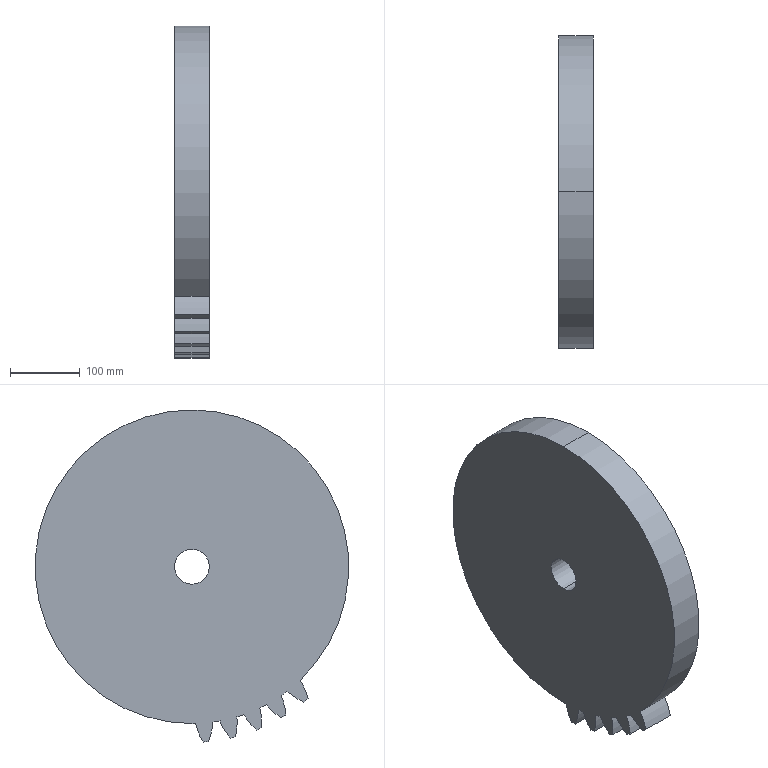Part | SolidWorks | features ICE 2, BaseBody 1 | 1 solid | 26 faces | box 50 x 449.998 x 476.498 mm | volume 7974553 mm3 | cylinder 24 | plane 2 | commonest cylinder face diameters 192 x10 449.998 x7 504 x5 50 x2
STEP:
#1=CARTESIAN_POINT('',(50.,0.,25.));
#2=VERTEX_POINT('',#1);
#3=CARTESIAN_POINT('',(50.,0.,-25.));
#4=VERTEX_POINT('',#3);
#5=CARTESIAN_POINT('',(50.,0.,0.));
#6=DIRECTION('',(1.,0.,0.));
#7=DIRECTION('',(0.,0.,1.));
#8=AXIS2_PLACEMENT_3D('',#5,#6,#7);
#9=CIRCLE('',#8,25.);
#10=EDGE_CURVE('',#2,#4,#9,.T.);
#11=ORIENTED_EDGE('',*,*,#10,.T.);
#12=CARTESIAN_POINT('',(0.,0.,-25.));
#13=VERTEX_POINT('',#12);
#14=CARTESIAN_POINT('',(50.,0.,-25.));
#15=DIRECTION('',(-1.,0.,0.));
#16=VECTOR('',#15,1000.);
#17=LINE('',#14,#16);
#18=EDGE_CURVE('',#4,#13,#17,.T.);
#19=ORIENTED_EDGE('',*,*,#18,.T.);
#20=CARTESIAN_POINT('',(0.,0.,25.));
#21=VERTEX_POINT('',#20);
#22=CARTESIAN_POINT('',(0.,0.,0.));
#23=DIRECTION('',(-1.,0.,0.));
#24=DIRECTION('',(0.,0.,1.));
#25=AXIS2_PLACEMENT_3D('',#22,#23,#24);
#26=CIRCLE('',#25,25.);
#27=EDGE_CURVE('',#13,#21,#26,.T.);
#28=ORIENTED_EDGE('',*,*,#27,.T.);
#29=CARTESIAN_POINT('',(50.,0.,25.));
#30=DIRECTION('',(-1.,0.,0.));
#31=VECTOR('',#30,1000.);
#32=LINE('',#29,#31);
#33=EDGE_CURVE('',#2,#21,#32,.T.);
#34=ORIENTED_EDGE('',*,*,#33,.F.);
#35=EDGE_LOOP('',(#11,#19,#28,#34));
#36=FACE_OUTER_BOUND('',#35,.T.);
#37=CARTESIAN_POINT('',(50.,0.,0.));
#38=DIRECTION('',(-1.,0.,0.));
#39=DIRECTION('',(0.,0.,1.));
#40=AXIS2_PLACEMENT_3D('',#37,#38,#39);
#41=CYLINDRICAL_SURFACE('',#40,25.);
#42=ADVANCED_FACE('',(#36),#41,.F.);
#43=CARTESIAN_POINT('',(50.,0.,224.999));
#44=VERTEX_POINT('',#43);
#45=CARTESIAN_POINT('',(50.,0.,-224.999));
#46=VERTEX_POINT('',#45);
#47=CARTESIAN_POINT('',(50.,0.,0.));
#48=DIRECTION('',(-1.,0.,0.));
#49=DIRECTION('',(0.,0.,-1.));
#50=AXIS2_PLACEMENT_3D('',#47,#48,#49);
#51=CIRCLE('',#50,224.999);
#52=EDGE_CURVE('',#44,#46,#51,.T.);
#53=ORIENTED_EDGE('',*,*,#52,.T.);
#54=CARTESIAN_POINT('',(0.,0.,-224.999));
#55=VERTEX_POINT('',#54);
#56=CARTESIAN_POINT('',(50.,0.,-224.999));
#57=DIRECTION('',(-1.,0.,0.));
#58=VECTOR('',#57,1000.);
#59=LINE('',#56,#58);
#60=EDGE_CURVE('',#46,#55,#59,.T.);
#61=ORIENTED_EDGE('',*,*,#60,.T.);
#62=CARTESIAN_POINT('',(0.,0.,224.999));
#63=VERTEX_POINT('',#62);
#64=CARTESIAN_POINT('',(0.,0.,0.));
#65=DIRECTION('',(-1.,0.,0.));
#66=DIRECTION('',(0.,0.,-1.));
#67=AXIS2_PLACEMENT_3D('',#64,#65,#66);
#68=CIRCLE('',#67,224.999);
#69=EDGE_CURVE('',#63,#55,#68,.T.);
#70=ORIENTED_EDGE('',*,*,#69,.F.);
#71=CARTESIAN_POINT('',(50.,0.,224.999));
#72=DIRECTION('',(-1.,0.,0.));
#73=VECTOR('',#72,1000.);
#74=LINE('',#71,#73);
#75=EDGE_CURVE('',#44,#63,#74,.T.);
#76=ORIENTED_EDGE('',*,*,#75,.F.);
#77=EDGE_LOOP('',(#53,#61,#70,#76));
#78=FACE_OUTER_BOUND('',#77,.T.);
#79=CARTESIAN_POINT('',(50.,0.,0.));
#80=DIRECTION('',(-1.,0.,0.));
#81=DIRECTION('',(0.,0.,1.));
#82=AXIS2_PLACEMENT_3D('',#79,#80,#81);
#83=CYLINDRICAL_SURFACE('',#82,224.999);
#84=ADVANCED_FACE('',(#78),#83,.T.);
#85=CARTESIAN_POINT('',(50.,-155.378,-162.734));
#86=VERTEX_POINT('',#85);
#87=CARTESIAN_POINT('',(50.,0.,0.));
#88=DIRECTION('',(-1.,0.,0.));
#89=DIRECTION('',(0.,0.,-1.));
#90=AXIS2_PLACEMENT_3D('',#87,#88,#89);
#91=CIRCLE('',#90,224.999);
#92=EDGE_CURVE('',#86,#44,#91,.T.);
#93=ORIENTED_EDGE('',*,*,#92,.T.);
#94=ORIENTED_EDGE('',*,*,#75,.T.);
#95=CARTESIAN_POINT('',(0.,-155.378,-162.734));
#96=VERTEX_POINT('',#95);
#97=CARTESIAN_POINT('',(0.,0.,0.));
#98=DIRECTION('',(-1.,0.,0.));
#99=DIRECTION('',(0.,0.,-1.));
#100=AXIS2_PLACEMENT_3D('',#97,#98,#99);
#101=CIRCLE('',#100,224.999);
#102=EDGE_CURVE('',#96,#63,#101,.T.);
#103=ORIENTED_EDGE('',*,*,#102,.F.);
#104=CARTESIAN_POINT('',(50.,-155.378,-162.734));
#105=DIRECTION('',(-1.,0.,0.));
#106=VECTOR('',#105,1000.);
#107=LINE('',#104,#106);
#108=EDGE_CURVE('',#86,#96,#107,.T.);
#109=ORIENTED_EDGE('',*,*,#108,.F.);
#110=EDGE_LOOP('',(#93,#94,#103,#109));
#111=FACE_OUTER_BOUND('',#110,.T.);
#112=CARTESIAN_POINT('',(50.,0.,0.));
#113=DIRECTION('',(-1.,0.,0.));
#114=DIRECTION('',(0.,0.,1.));
#115=AXIS2_PLACEMENT_3D('',#112,#113,#114);
#116=CYLINDRICAL_SURFACE('',#115,224.999);
#117=ADVANCED_FACE('',(#111),#116,.T.);
#118=ORIENTED_EDGE('',*,*,#10,.F.);
#119=CARTESIAN_POINT('',(50.,0.,0.));
#120=DIRECTION('',(1.,0.,0.));
#121=DIRECTION('',(0.,0.,1.));
#122=AXIS2_PLACEMENT_3D('',#119,#120,#121);
#123=CIRCLE('',#122,25.);
#124=EDGE_CURVE('',#4,#2,#123,.T.);
#125=ORIENTED_EDGE('',*,*,#124,.F.);
#126=EDGE_LOOP('',(#118,#125));
#127=FACE_BOUND('',#126,.T.);
#128=ORIENTED_EDGE('',*,*,#92,.F.);
#129=CARTESIAN_POINT('',(50.,-166.611,-189.062));
#130=VERTEX_POINT('',#129);
#131=CARTESIAN_POINT('',(50.,-73.683,-213.15));
#132=DIRECTION('',(-1.,0.,0.));
#133=DIRECTION('',(0.,-0.7071,0.7071));
#134=AXIS2_PLACEMENT_3D('',#131,#132,#133);
#135=CIRCLE('',#134,96.);
#136=EDGE_CURVE('',#130,#86,#135,.T.);
#137=ORIENTED_EDGE('',*,*,#136,.F.);
#138=CARTESIAN_POINT('',(50.,-160.671,-194.136));
#139=VERTEX_POINT('',#138);
#140=CARTESIAN_POINT('',(50.,0.,0.));
#141=DIRECTION('',(-1.,0.,0.));
#142=DIRECTION('',(0.,0.,1.));
#143=AXIS2_PLACEMENT_3D('',#140,#141,#142);
#144=CIRCLE('',#143,252.);
#145=EDGE_CURVE('',#139,#130,#144,.T.);
#146=ORIENTED_EDGE('',*,*,#145,.F.);
#147=CARTESIAN_POINT('',(50.,-136.423,-178.922));
#148=VERTEX_POINT('',#147);
#149=CARTESIAN_POINT('',(50.,-198.999,-106.119));
#150=DIRECTION('',(-1.,0.,0.));
#151=DIRECTION('',(0.,-0.809,0.5878));
#152=AXIS2_PLACEMENT_3D('',#149,#150,#151);
#153=CIRCLE('',#152,96.);
#154=EDGE_CURVE('',#148,#139,#153,.T.);
#155=ORIENTED_EDGE('',*,*,#154,.F.);
#156=CARTESIAN_POINT('',(50.,-128.008,-185.036));
#157=VERTEX_POINT('',#156);
#158=CARTESIAN_POINT('',(50.,0.,0.));
#159=DIRECTION('',(-1.,0.,0.));
#160=DIRECTION('',(0.,-0.809,0.5878));
#161=AXIS2_PLACEMENT_3D('',#158,#159,#160);
#162=CIRCLE('',#161,224.999);
#163=EDGE_CURVE('',#157,#148,#162,.T.);
#164=ORIENTED_EDGE('',*,*,#163,.F.);
#165=CARTESIAN_POINT('',(50.,-134.984,-212.799));
#166=VERTEX_POINT('',#165);
#167=CARTESIAN_POINT('',(50.,-39.431,-222.052));
#168=DIRECTION('',(-1.,0.,0.));
#169=DIRECTION('',(0.,-0.809,0.5878));
#170=AXIS2_PLACEMENT_3D('',#167,#168,#169);
#171=CIRCLE('',#170,96.);
#172=EDGE_CURVE('',#166,#157,#171,.T.);
#173=ORIENTED_EDGE('',*,*,#172,.F.);
#174=CARTESIAN_POINT('',(50.,-128.323,-216.88));
#175=VERTEX_POINT('',#174);
#176=CARTESIAN_POINT('',(50.,0.,0.));
#177=DIRECTION('',(-1.,0.,0.));
#178=DIRECTION('',(0.,0.,1.));
#179=AXIS2_PLACEMENT_3D('',#176,#177,#178);
#180=CIRCLE('',#179,252.);
#181=EDGE_CURVE('',#175,#166,#180,.T.);
#182=ORIENTED_EDGE('',*,*,#181,.F.);
#183=CARTESIAN_POINT('',(50.,-106.754,-198.061));
#184=VERTEX_POINT('',#183);
#185=CARTESIAN_POINT('',(50.,-179.949,-135.943));
#186=DIRECTION('',(-1.,0.,0.));
#187=DIRECTION('',(0.,-0.891,0.454));
#188=AXIS2_PLACEMENT_3D('',#185,#186,#187);
#189=CIRCLE('',#188,96.);
#190=EDGE_CURVE('',#184,#175,#189,.T.);
#191=ORIENTED_EDGE('',*,*,#190,.F.);
#192=CARTESIAN_POINT('',(50.,-97.486,-202.783));
#193=VERTEX_POINT('',#192);
#194=CARTESIAN_POINT('',(50.,0.,0.));
#195=DIRECTION('',(-1.,0.,0.));
#196=DIRECTION('',(0.,-0.891,0.454));
#197=AXIS2_PLACEMENT_3D('',#194,#195,#196);
#198=CIRCLE('',#197,224.999);
#199=EDGE_CURVE('',#193,#184,#198,.T.);
#200=ORIENTED_EDGE('',*,*,#199,.F.);
#201=CARTESIAN_POINT('',(50.,-100.033,-231.295));
#202=VERTEX_POINT('',#201);
#203=CARTESIAN_POINT('',(50.,-4.209,-225.487));
#204=DIRECTION('',(-1.,0.,0.));
#205=DIRECTION('',(0.,-0.891,0.454));
#206=AXIS2_PLACEMENT_3D('',#203,#204,#205);
#207=CIRCLE('',#206,96.);
#208=EDGE_CURVE('',#202,#193,#207,.T.);
#209=ORIENTED_EDGE('',*,*,#208,.F.);
#210=CARTESIAN_POINT('',(50.,-92.816,-234.284));
#211=VERTEX_POINT('',#210);
#212=CARTESIAN_POINT('',(50.,0.,0.));
#213=DIRECTION('',(-1.,0.,0.));
#214=DIRECTION('',(0.,0.,1.));
#215=AXIS2_PLACEMENT_3D('',#212,#213,#214);
#216=CIRCLE('',#215,252.);
#217=EDGE_CURVE('',#211,#202,#216,.T.);
#218=ORIENTED_EDGE('',*,*,#217,.F.);
#219=CARTESIAN_POINT('',(50.,-74.456,-212.322));
#220=VERTEX_POINT('',#219);
#221=CARTESIAN_POINT('',(50.,-156.467,-162.42));
#222=DIRECTION('',(-1.,0.,0.));
#223=DIRECTION('',(0.,-0.9511,0.309));
#224=AXIS2_PLACEMENT_3D('',#221,#222,#223);
#225=CIRCLE('',#224,96.);
#226=EDGE_CURVE('',#220,#211,#225,.T.);
#227=ORIENTED_EDGE('',*,*,#226,.F.);
#228=CARTESIAN_POINT('',(50.,-64.563,-215.537));
#229=VERTEX_POINT('',#228);
#230=CARTESIAN_POINT('',(50.,0.,0.));
#231=DIRECTION('',(-1.,0.,0.));
#232=DIRECTION('',(0.,-0.9511,0.309));
#233=AXIS2_PLACEMENT_3D('',#230,#231,#232);
#234=CIRCLE('',#233,224.999);
#235=EDGE_CURVE('',#229,#220,#234,.T.);
#236=ORIENTED_EDGE('',*,*,#235,.F.);
#237=CARTESIAN_POINT('',(50.,-62.619,-244.096));
#238=VERTEX_POINT('',#237);
#239=CARTESIAN_POINT('',(50.,31.117,-223.369));
#240=DIRECTION('',(-1.,0.,0.));
#241=DIRECTION('',(0.,-0.9511,0.309));
#242=AXIS2_PLACEMENT_3D('',#239,#240,#241);
#243=CIRCLE('',#242,96.);
#244=EDGE_CURVE('',#238,#229,#243,.T.);
#245=ORIENTED_EDGE('',*,*,#244,.F.);
#246=CARTESIAN_POINT('',(50.,-55.023,-245.92));
#247=VERTEX_POINT('',#246);
#248=CARTESIAN_POINT('',(50.,0.,0.));
#249=DIRECTION('',(-1.,0.,0.));
#250=DIRECTION('',(0.,0.,1.));
#251=AXIS2_PLACEMENT_3D('',#248,#249,#250);
#252=CIRCLE('',#251,252.);
#253=EDGE_CURVE('',#247,#238,#252,.T.);
#254=ORIENTED_EDGE('',*,*,#253,.F.);
#255=CARTESIAN_POINT('',(50.,-40.325,-221.356));
#256=VERTEX_POINT('',#255);
#257=CARTESIAN_POINT('',(50.,-129.133,-184.897));
#258=DIRECTION('',(-1.,0.,0.));
#259=DIRECTION('',(0.,-0.9877,0.1564));
#260=AXIS2_PLACEMENT_3D('',#257,#258,#259);
#261=CIRCLE('',#260,96.);
#262=EDGE_CURVE('',#256,#247,#261,.T.);
#263=ORIENTED_EDGE('',*,*,#262,.F.);
#264=CARTESIAN_POINT('',(50.,-30.051,-222.983));
#265=VERTEX_POINT('',#264);
#266=CARTESIAN_POINT('',(50.,0.,0.));
#267=DIRECTION('',(-1.,0.,0.));
#268=DIRECTION('',(0.,-0.9877,0.1564));
#269=AXIS2_PLACEMENT_3D('',#266,#267,#268);
#270=CIRCLE('',#269,224.999);
#271=EDGE_CURVE('',#265,#256,#270,.T.);
#272=ORIENTED_EDGE('',*,*,#271,.F.);
#273=CARTESIAN_POINT('',(50.,-23.663,-250.887));
#274=VERTEX_POINT('',#273);
#275=CARTESIAN_POINT('',(50.,65.676,-215.752));
#276=DIRECTION('',(-1.,0.,0.));
#277=DIRECTION('',(0.,-0.9877,0.1564));
#278=AXIS2_PLACEMENT_3D('',#275,#276,#277);
#279=CIRCLE('',#278,96.);
#280=EDGE_CURVE('',#274,#265,#279,.T.);
#281=ORIENTED_EDGE('',*,*,#280,.F.);
#282=CARTESIAN_POINT('',(50.,-15.875,-251.499));
#283=VERTEX_POINT('',#282);
#284=CARTESIAN_POINT('',(50.,0.,0.));
#285=DIRECTION('',(-1.,0.,0.));
#286=DIRECTION('',(0.,0.,1.));
#287=AXIS2_PLACEMENT_3D('',#284,#285,#286);
#288=CIRCLE('',#287,252.);
#289=EDGE_CURVE('',#283,#274,#288,.T.);
#290=ORIENTED_EDGE('',*,*,#289,.F.);
#291=CARTESIAN_POINT('',(50.,-5.201,-224.939));
#292=VERTEX_POINT('',#291);
#293=CARTESIAN_POINT('',(50.,-98.618,-202.821));
#294=DIRECTION('',(-1.,0.,0.));
#295=DIRECTION('',(0.,-1.,0.));
#296=AXIS2_PLACEMENT_3D('',#293,#294,#295);
#297=CIRCLE('',#296,96.);
#298=EDGE_CURVE('',#292,#283,#297,.T.);
#299=ORIENTED_EDGE('',*,*,#298,.F.);
#300=CARTESIAN_POINT('',(50.,0.,0.));
#301=DIRECTION('',(-1.,0.,0.));
#302=DIRECTION('',(0.,0.,-1.));
#303=AXIS2_PLACEMENT_3D('',#300,#301,#302);
#304=CIRCLE('',#303,224.999);
#305=EDGE_CURVE('',#46,#292,#304,.T.);
#306=ORIENTED_EDGE('',*,*,#305,.F.);
#307=ORIENTED_EDGE('',*,*,#52,.F.);
#308=EDGE_LOOP('',(#128,#137,#146,#155,#164,#173,#182,#191,#200,#209,#218,#227,#236,#245,#254,#263,#272,#281,#290,#299,#306,#307));
#309=FACE_OUTER_BOUND('',#308,.T.);
#310=CARTESIAN_POINT('',(50.,0.,0.));
#311=DIRECTION('',(-1.,0.,0.));
#312=DIRECTION('',(0.,0.,1.));
#313=AXIS2_PLACEMENT_3D('',#310,#311,#312);
#314=PLANE('',#313);
#315=ADVANCED_FACE('',(#127,#309),#314,.F.);
#316=CARTESIAN_POINT('',(0.,-160.671,-194.136));
#317=VERTEX_POINT('',#316);
#318=CARTESIAN_POINT('',(25.,-160.671,-194.136));
#319=DIRECTION('',(-1.,0.,0.));
#320=VECTOR('',#319,1000.);
#321=LINE('',#318,#320);
#322=EDGE_CURVE('',#139,#317,#321,.T.);
#323=ORIENTED_EDGE('',*,*,#322,.F.);
#324=ORIENTED_EDGE('',*,*,#145,.T.);
#325=CARTESIAN_POINT('',(0.,-166.611,-189.062));
#326=VERTEX_POINT('',#325);
#327=CARTESIAN_POINT('',(25.,-166.611,-189.062));
#328=DIRECTION('',(1.,0.,0.));
#329=VECTOR('',#328,1000.);
#330=LINE('',#327,#329);
#331=EDGE_CURVE('',#326,#130,#330,.T.);
#332=ORIENTED_EDGE('',*,*,#331,.F.);
#333=CARTESIAN_POINT('',(0.,0.,0.));
#334=DIRECTION('',(-1.,0.,0.));
#335=DIRECTION('',(0.,0.,1.));
#336=AXIS2_PLACEMENT_3D('',#333,#334,#335);
#337=CIRCLE('',#336,252.);
#338=EDGE_CURVE('',#317,#326,#337,.T.);
#339=ORIENTED_EDGE('',*,*,#338,.F.);
#340=EDGE_LOOP('',(#323,#324,#332,#339));
#341=FACE_OUTER_BOUND('',#340,.T.);
#342=CARTESIAN_POINT('',(-10.,0.,0.));
#343=DIRECTION('',(-1.,0.,0.));
#344=DIRECTION('',(0.,0.,1.));
#345=AXIS2_PLACEMENT_3D('',#342,#343,#344);
#346=CYLINDRICAL_SURFACE('',#345,252.);
#347=ADVANCED_FACE('',(#341),#346,.T.);
#348=CARTESIAN_POINT('',(0.,-134.984,-212.799));
#349=VERTEX_POINT('',#348);
#350=CARTESIAN_POINT('',(25.,-134.984,-212.799));
#351=DIRECTION('',(1.,0.,0.));
#352=VECTOR('',#351,1000.);
#353=LINE('',#350,#352);
#354=EDGE_CURVE('',#349,#166,#353,.T.);
#355=ORIENTED_EDGE('',*,*,#354,.F.);
#356=CARTESIAN_POINT('',(0.,-128.323,-216.88));
#357=VERTEX_POINT('',#356);
#358=CARTESIAN_POINT('',(0.,0.,0.));
#359=DIRECTION('',(-1.,0.,0.));
#360=DIRECTION('',(0.,0.,1.));
#361=AXIS2_PLACEMENT_3D('',#358,#359,#360);
#362=CIRCLE('',#361,252.);
#363=EDGE_CURVE('',#357,#349,#362,.T.);
#364=ORIENTED_EDGE('',*,*,#363,.F.);
#365=CARTESIAN_POINT('',(25.,-128.323,-216.88));
#366=DIRECTION('',(-1.,0.,0.));
#367=VECTOR('',#366,1000.);
#368=LINE('',#365,#367);
#369=EDGE_CURVE('',#175,#357,#368,.T.);
#370=ORIENTED_EDGE('',*,*,#369,.F.);
#371=ORIENTED_EDGE('',*,*,#181,.T.);
#372=EDGE_LOOP('',(#355,#364,#370,#371));
#373=FACE_OUTER_BOUND('',#372,.T.);
#374=CARTESIAN_POINT('',(-10.,0.,0.));
#375=DIRECTION('',(-1.,0.,0.));
#376=DIRECTION('',(0.,0.,1.));
#377=AXIS2_PLACEMENT_3D('',#374,#375,#376);
#378=CYLINDRICAL_SURFACE('',#377,252.);
#379=ADVANCED_FACE('',(#373),#378,.T.);
#380=CARTESIAN_POINT('',(0.,-100.033,-231.295));
#381=VERTEX_POINT('',#380);
#382=CARTESIAN_POINT('',(25.,-100.033,-231.295));
#383=DIRECTION('',(1.,0.,0.));
#384=VECTOR('',#383,1000.);
#385=LINE('',#382,#384);
#386=EDGE_CURVE('',#381,#202,#385,.T.);
#387=ORIENTED_EDGE('',*,*,#386,.F.);
#388=CARTESIAN_POINT('',(0.,-92.816,-234.284));
#389=VERTEX_POINT('',#388);
#390=CARTESIAN_POINT('',(0.,0.,0.));
#391=DIRECTION('',(-1.,0.,0.));
#392=DIRECTION('',(0.,0.,1.));
#393=AXIS2_PLACEMENT_3D('',#390,#391,#392);
#394=CIRCLE('',#393,252.);
#395=EDGE_CURVE('',#389,#381,#394,.T.);
#396=ORIENTED_EDGE('',*,*,#395,.F.);
#397=CARTESIAN_POINT('',(25.,-92.816,-234.284));
#398=DIRECTION('',(-1.,0.,0.));
#399=VECTOR('',#398,1000.);
#400=LINE('',#397,#399);
#401=EDGE_CURVE('',#211,#389,#400,.T.);
#402=ORIENTED_EDGE('',*,*,#401,.F.);
#403=ORIENTED_EDGE('',*,*,#217,.T.);
#404=EDGE_LOOP('',(#387,#396,#402,#403));
#405=FACE_OUTER_BOUND('',#404,.T.);
#406=CARTESIAN_POINT('',(-10.,0.,0.));
#407=DIRECTION('',(-1.,0.,0.));
#408=DIRECTION('',(0.,0.,1.));
#409=AXIS2_PLACEMENT_3D('',#406,#407,#408);
#410=CYLINDRICAL_SURFACE('',#409,252.);
#411=ADVANCED_FACE('',(#405),#410,.T.);
#412=CARTESIAN_POINT('',(0.,-62.619,-244.096));
#413=VERTEX_POINT('',#412);
#414=CARTESIAN_POINT('',(25.,-62.619,-244.096));
#415=DIRECTION('',(1.,0.,0.));
#416=VECTOR('',#415,1000.);
#417=LINE('',#414,#416);
#418=EDGE_CURVE('',#413,#238,#417,.T.);
#419=ORIENTED_EDGE('',*,*,#418,.F.);
#420=CARTESIAN_POINT('',(0.,-55.023,-245.92));
#421=VERTEX_POINT('',#420);
#422=CARTESIAN_POINT('',(0.,0.,0.));
#423=DIRECTION('',(-1.,0.,0.));
#424=DIRECTION('',(0.,0.,1.));
#425=AXIS2_PLACEMENT_3D('',#422,#423,#424);
#426=CIRCLE('',#425,252.);
#427=EDGE_CURVE('',#421,#413,#426,.T.);
#428=ORIENTED_EDGE('',*,*,#427,.F.);
#429=CARTESIAN_POINT('',(25.,-55.023,-245.92));
#430=DIRECTION('',(-1.,0.,0.));
#431=VECTOR('',#430,1000.);
#432=LINE('',#429,#431);
#433=EDGE_CURVE('',#247,#421,#432,.T.);
#434=ORIENTED_EDGE('',*,*,#433,.F.);
#435=ORIENTED_EDGE('',*,*,#253,.T.);
#436=EDGE_LOOP('',(#419,#428,#434,#435));
#437=FACE_OUTER_BOUND('',#436,.T.);
#438=CARTESIAN_POINT('',(-10.,0.,0.));
#439=DIRECTION('',(-1.,0.,0.));
#440=DIRECTION('',(0.,0.,1.));
#441=AXIS2_PLACEMENT_3D('',#438,#439,#440);
#442=CYLINDRICAL_SURFACE('',#441,252.);
#443=ADVANCED_FACE('',(#437),#442,.T.);
#444=CARTESIAN_POINT('',(0.,-23.663,-250.887));
#445=VERTEX_POINT('',#444);
#446=CARTESIAN_POINT('',(25.,-23.663,-250.887));
#447=DIRECTION('',(1.,0.,0.));
#448=VECTOR('',#447,1000.);
#449=LINE('',#446,#448);
#450=EDGE_CURVE('',#445,#274,#449,.T.);
#451=ORIENTED_EDGE('',*,*,#450,.F.);
#452=CARTESIAN_POINT('',(0.,-15.875,-251.499));
#453=VERTEX_POINT('',#452);
#454=CARTESIAN_POINT('',(0.,0.,0.));
#455=DIRECTION('',(-1.,0.,0.));
#456=DIRECTION('',(0.,0.,1.));
#457=AXIS2_PLACEMENT_3D('',#454,#455,#456);
#458=CIRCLE('',#457,252.);
#459=EDGE_CURVE('',#453,#445,#458,.T.);
#460=ORIENTED_EDGE('',*,*,#459,.F.);
#461=CARTESIAN_POINT('',(25.,-15.875,-251.499));
#462=DIRECTION('',(-1.,0.,0.));
#463=VECTOR('',#462,1000.);
#464=LINE('',#461,#463);
#465=EDGE_CURVE('',#283,#453,#464,.T.);
#466=ORIENTED_EDGE('',*,*,#465,.F.);
#467=ORIENTED_EDGE('',*,*,#289,.T.);
#468=EDGE_LOOP('',(#451,#460,#466,#467));
#469=FACE_OUTER_BOUND('',#468,.T.);
#470=CARTESIAN_POINT('',(-10.,0.,0.));
#471=DIRECTION('',(-1.,0.,0.));
#472=DIRECTION('',(0.,0.,1.));
#473=AXIS2_PLACEMENT_3D('',#470,#471,#472);
#474=CYLINDRICAL_SURFACE('',#473,252.);
#475=ADVANCED_FACE('',(#469),#474,.T.);
#476=CARTESIAN_POINT('',(0.,-73.683,-213.15));
#477=DIRECTION('',(1.,0.,0.));
#478=DIRECTION('',(0.,0.,-1.));
#479=AXIS2_PLACEMENT_3D('',#476,#477,#478);
#480=CIRCLE('',#479,96.);
#481=EDGE_CURVE('',#96,#326,#480,.T.);
#482=ORIENTED_EDGE('',*,*,#481,.F.);
#483=ORIENTED_EDGE('',*,*,#102,.T.);
#484=ORIENTED_EDGE('',*,*,#69,.T.);
#485=CARTESIAN_POINT('',(0.,-5.201,-224.939));
#486=VERTEX_POINT('',#485);
#487=CARTESIAN_POINT('',(0.,0.,0.));
#488=DIRECTION('',(-1.,0.,0.));
#489=DIRECTION('',(0.,0.,-1.));
#490=AXIS2_PLACEMENT_3D('',#487,#488,#489);
#491=CIRCLE('',#490,224.999);
#492=EDGE_CURVE('',#55,#486,#491,.T.);
#493=ORIENTED_EDGE('',*,*,#492,.T.);
#494=CARTESIAN_POINT('',(0.,-98.618,-202.821));
#495=DIRECTION('',(-1.,0.,0.));
#496=DIRECTION('',(0.,-1.,0.));
#497=AXIS2_PLACEMENT_3D('',#494,#495,#496);
#498=CIRCLE('',#497,96.);
#499=EDGE_CURVE('',#486,#453,#498,.T.);
#500=ORIENTED_EDGE('',*,*,#499,.T.);
#501=ORIENTED_EDGE('',*,*,#459,.T.);
#502=CARTESIAN_POINT('',(0.,-30.051,-222.983));
#503=VERTEX_POINT('',#502);
#504=CARTESIAN_POINT('',(0.,65.676,-215.752));
#505=DIRECTION('',(1.,0.,0.));
#506=DIRECTION('',(0.,0.,-1.));
#507=AXIS2_PLACEMENT_3D('',#504,#505,#506);
#508=CIRCLE('',#507,96.);
#509=EDGE_CURVE('',#503,#445,#508,.T.);
#510=ORIENTED_EDGE('',*,*,#509,.F.);
#511=CARTESIAN_POINT('',(0.,-40.325,-221.356));
#512=VERTEX_POINT('',#511);
#513=CARTESIAN_POINT('',(0.,0.,0.));
#514=DIRECTION('',(-1.,0.,0.));
#515=DIRECTION('',(0.,-0.9877,0.1564));
#516=AXIS2_PLACEMENT_3D('',#513,#514,#515);
#517=CIRCLE('',#516,224.999);
#518=EDGE_CURVE('',#503,#512,#517,.T.);
#519=ORIENTED_EDGE('',*,*,#518,.T.);
#520=CARTESIAN_POINT('',(0.,-129.133,-184.897));
#521=DIRECTION('',(-1.,0.,0.));
#522=DIRECTION('',(0.,-0.9877,0.1564));
#523=AXIS2_PLACEMENT_3D('',#520,#521,#522);
#524=CIRCLE('',#523,96.);
#525=EDGE_CURVE('',#512,#421,#524,.T.);
#526=ORIENTED_EDGE('',*,*,#525,.T.);
#527=ORIENTED_EDGE('',*,*,#427,.T.);
#528=CARTESIAN_POINT('',(0.,-64.563,-215.537));
#529=VERTEX_POINT('',#528);
#530=CARTESIAN_POINT('',(0.,31.117,-223.369));
#531=DIRECTION('',(1.,0.,0.));
#532=DIRECTION('',(0.,0.,-1.));
#533=AXIS2_PLACEMENT_3D('',#530,#531,#532);
#534=CIRCLE('',#533,96.);
#535=EDGE_CURVE('',#529,#413,#534,.T.);
#536=ORIENTED_EDGE('',*,*,#535,.F.);
#537=CARTESIAN_POINT('',(0.,-74.456,-212.322));
#538=VERTEX_POINT('',#537);
#539=CARTESIAN_POINT('',(0.,0.,0.));
#540=DIRECTION('',(-1.,0.,0.));
#541=DIRECTION('',(0.,-0.9511,0.309));
#542=AXIS2_PLACEMENT_3D('',#539,#540,#541);
#543=CIRCLE('',#542,224.999);
#544=EDGE_CURVE('',#529,#538,#543,.T.);
#545=ORIENTED_EDGE('',*,*,#544,.T.);
#546=CARTESIAN_POINT('',(0.,-156.467,-162.42));
#547=DIRECTION('',(-1.,0.,0.));
#548=DIRECTION('',(0.,-0.9511,0.309));
#549=AXIS2_PLACEMENT_3D('',#546,#547,#548);
#550=CIRCLE('',#549,96.);
#551=EDGE_CURVE('',#538,#389,#550,.T.);
#552=ORIENTED_EDGE('',*,*,#551,.T.);
#553=ORIENTED_EDGE('',*,*,#395,.T.);
#554=CARTESIAN_POINT('',(0.,-97.486,-202.783));
#555=VERTEX_POINT('',#554);
#556=CARTESIAN_POINT('',(0.,-4.209,-225.487));
#557=DIRECTION('',(1.,0.,0.));
#558=DIRECTION('',(0.,0.,-1.));
#559=AXIS2_PLACEMENT_3D('',#556,#557,#558);
#560=CIRCLE('',#559,96.);
#561=EDGE_CURVE('',#555,#381,#560,.T.);
#562=ORIENTED_EDGE('',*,*,#561,.F.);
#563=CARTESIAN_POINT('',(0.,-106.754,-198.061));
#564=VERTEX_POINT('',#563);
#565=CARTESIAN_POINT('',(0.,0.,0.));
#566=DIRECTION('',(-1.,0.,0.));
#567=DIRECTION('',(0.,-0.891,0.454));
#568=AXIS2_PLACEMENT_3D('',#565,#566,#567);
#569=CIRCLE('',#568,224.999);
#570=EDGE_CURVE('',#555,#564,#569,.T.);
#571=ORIENTED_EDGE('',*,*,#570,.T.);
#572=CARTESIAN_POINT('',(0.,-179.949,-135.943));
#573=DIRECTION('',(-1.,0.,0.));
#574=DIRECTION('',(0.,-0.891,0.454));
#575=AXIS2_PLACEMENT_3D('',#572,#573,#574);
#576=CIRCLE('',#575,96.);
#577=EDGE_CURVE('',#564,#357,#576,.T.);
#578=ORIENTED_EDGE('',*,*,#577,.T.);
#579=ORIENTED_EDGE('',*,*,#363,.T.);
#580=CARTESIAN_POINT('',(0.,-128.008,-185.036));
#581=VERTEX_POINT('',#580);
#582=CARTESIAN_POINT('',(0.,-39.431,-222.052));
#583=DIRECTION('',(1.,0.,0.));
#584=DIRECTION('',(0.,0.,-1.));
#585=AXIS2_PLACEMENT_3D('',#582,#583,#584);
#586=CIRCLE('',#585,96.);
#587=EDGE_CURVE('',#581,#349,#586,.T.);
#588=ORIENTED_EDGE('',*,*,#587,.F.);
#589=CARTESIAN_POINT('',(0.,-136.423,-178.922));
#590=VERTEX_POINT('',#589);
#591=CARTESIAN_POINT('',(0.,0.,0.));
#592=DIRECTION('',(-1.,0.,0.));
#593=DIRECTION('',(0.,-0.809,0.5878));
#594=AXIS2_PLACEMENT_3D('',#591,#592,#593);
#595=CIRCLE('',#594,224.999);
#596=EDGE_CURVE('',#581,#590,#595,.T.);
#597=ORIENTED_EDGE('',*,*,#596,.T.);
#598=CARTESIAN_POINT('',(0.,-198.999,-106.119));
#599=DIRECTION('',(-1.,0.,0.));
#600=DIRECTION('',(0.,-0.809,0.5878));
#601=AXIS2_PLACEMENT_3D('',#598,#599,#600);
#602=CIRCLE('',#601,96.);
#603=EDGE_CURVE('',#590,#317,#602,.T.);
#604=ORIENTED_EDGE('',*,*,#603,.T.);
#605=ORIENTED_EDGE('',*,*,#338,.T.);
#606=EDGE_LOOP('',(#482,#483,#484,#493,#500,#501,#510,#519,#526,#527,#536,#545,#552,#553,#562,#571,#578,#579,#588,#597,#604,#605));
#607=FACE_OUTER_BOUND('',#606,.T.);
#608=CARTESIAN_POINT('',(0.,0.,0.));
#609=DIRECTION('',(-1.,0.,0.));
#610=DIRECTION('',(0.,0.,1.));
#611=AXIS2_PLACEMENT_3D('',#608,#609,#610);
#612=CIRCLE('',#611,25.);
#613=EDGE_CURVE('',#21,#13,#612,.T.);
#614=ORIENTED_EDGE('',*,*,#613,.F.);
#615=ORIENTED_EDGE('',*,*,#27,.F.);
#616=EDGE_LOOP('',(#614,#615));
#617=FACE_BOUND('',#616,.T.);
#618=CARTESIAN_POINT('',(0.,0.,0.));
#619=DIRECTION('',(1.,0.,0.));
#620=DIRECTION('',(0.,0.,-1.));
#621=AXIS2_PLACEMENT_3D('',#618,#619,#620);
#622=PLANE('',#621);
#623=ADVANCED_FACE('',(#607,#617),#622,.F.);
#624=ORIENTED_EDGE('',*,*,#60,.F.);
#625=ORIENTED_EDGE('',*,*,#305,.T.);
#626=CARTESIAN_POINT('',(50.,-5.201,-224.939));
#627=DIRECTION('',(-1.,0.,0.));
#628=VECTOR('',#627,1000.);
#629=LINE('',#626,#628);
#630=EDGE_CURVE('',#292,#486,#629,.T.);
#631=ORIENTED_EDGE('',*,*,#630,.T.);
#632=ORIENTED_EDGE('',*,*,#492,.F.);
#633=EDGE_LOOP('',(#624,#625,#631,#632));
#634=FACE_OUTER_BOUND('',#633,.T.);
#635=CARTESIAN_POINT('',(50.,0.,0.));
#636=DIRECTION('',(-1.,0.,0.));
#637=DIRECTION('',(0.,0.,1.));
#638=AXIS2_PLACEMENT_3D('',#635,#636,#637);
#639=CYLINDRICAL_SURFACE('',#638,224.999);
#640=ADVANCED_FACE('',(#634),#639,.T.);
#641=ORIENTED_EDGE('',*,*,#465,.T.);
#642=ORIENTED_EDGE('',*,*,#499,.F.);
#643=ORIENTED_EDGE('',*,*,#630,.F.);
#644=ORIENTED_EDGE('',*,*,#298,.T.);
#645=EDGE_LOOP('',(#641,#642,#643,#644));
#646=FACE_OUTER_BOUND('',#645,.T.);
#647=CARTESIAN_POINT('',(50.,-98.618,-202.821));
#648=DIRECTION('',(-1.,0.,0.));
#649=DIRECTION('',(0.,0.,1.));
#650=AXIS2_PLACEMENT_3D('',#647,#648,#649);
#651=CYLINDRICAL_SURFACE('',#650,96.);
#652=ADVANCED_FACE('',(#646),#651,.T.);
#653=ORIENTED_EDGE('',*,*,#433,.T.);
#654=ORIENTED_EDGE('',*,*,#525,.F.);
#655=CARTESIAN_POINT('',(50.,-40.325,-221.356));
#656=DIRECTION('',(-1.,0.,0.));
#657=VECTOR('',#656,1000.);
#658=LINE('',#655,#657);
#659=EDGE_CURVE('',#256,#512,#658,.T.);
#660=ORIENTED_EDGE('',*,*,#659,.F.);
#661=ORIENTED_EDGE('',*,*,#262,.T.);
#662=EDGE_LOOP('',(#653,#654,#660,#661));
#663=FACE_OUTER_BOUND('',#662,.T.);
#664=CARTESIAN_POINT('',(50.,-129.133,-184.897));
#665=DIRECTION('',(-1.,0.,0.));
#666=DIRECTION('',(0.,0.,1.));
#667=AXIS2_PLACEMENT_3D('',#664,#665,#666);
#668=CYLINDRICAL_SURFACE('',#667,96.);
#669=ADVANCED_FACE('',(#663),#668,.T.);
#670=ORIENTED_EDGE('',*,*,#450,.T.);
#671=ORIENTED_EDGE('',*,*,#280,.T.);
#672=CARTESIAN_POINT('',(50.,-30.051,-222.983));
#673=DIRECTION('',(-1.,0.,0.));
#674=VECTOR('',#673,1000.);
#675=LINE('',#672,#674);
#676=EDGE_CURVE('',#265,#503,#675,.T.);
#677=ORIENTED_EDGE('',*,*,#676,.T.);
#678=ORIENTED_EDGE('',*,*,#509,.T.);
#679=EDGE_LOOP('',(#670,#671,#677,#678));
#680=FACE_OUTER_BOUND('',#679,.T.);
#681=CARTESIAN_POINT('',(50.,65.676,-215.752));
#682=DIRECTION('',(-1.,0.,0.));
#683=DIRECTION('',(0.,0.,1.));
#684=AXIS2_PLACEMENT_3D('',#681,#682,#683);
#685=CYLINDRICAL_SURFACE('',#684,96.);
#686=ADVANCED_FACE('',(#680),#685,.T.);
#687=ORIENTED_EDGE('',*,*,#518,.F.);
#688=ORIENTED_EDGE('',*,*,#676,.F.);
#689=ORIENTED_EDGE('',*,*,#271,.T.);
#690=ORIENTED_EDGE('',*,*,#659,.T.);
#691=EDGE_LOOP('',(#687,#688,#689,#690));
#692=FACE_OUTER_BOUND('',#691,.T.);
#693=CARTESIAN_POINT('',(50.,0.,0.));
#694=DIRECTION('',(-1.,0.,0.));
#695=DIRECTION('',(0.,0.,1.));
#696=AXIS2_PLACEMENT_3D('',#693,#694,#695);
#697=CYLINDRICAL_SURFACE('',#696,224.999);
#698=ADVANCED_FACE('',(#692),#697,.T.);
#699=ORIENTED_EDGE('',*,*,#401,.T.);
#700=ORIENTED_EDGE('',*,*,#551,.F.);
#701=CARTESIAN_POINT('',(50.,-74.456,-212.322));
#702=DIRECTION('',(-1.,0.,0.));
#703=VECTOR('',#702,1000.);
#704=LINE('',#701,#703);
#705=EDGE_CURVE('',#220,#538,#704,.T.);
#706=ORIENTED_EDGE('',*,*,#705,.F.);
#707=ORIENTED_EDGE('',*,*,#226,.T.);
#708=EDGE_LOOP('',(#699,#700,#706,#707));
#709=FACE_OUTER_BOUND('',#708,.T.);
#710=CARTESIAN_POINT('',(50.,-156.467,-162.42));
#711=DIRECTION('',(-1.,0.,0.));
#712=DIRECTION('',(0.,0.,1.));
#713=AXIS2_PLACEMENT_3D('',#710,#711,#712);
#714=CYLINDRICAL_SURFACE('',#713,96.);
#715=ADVANCED_FACE('',(#709),#714,.T.);
#716=ORIENTED_EDGE('',*,*,#418,.T.);
#717=ORIENTED_EDGE('',*,*,#244,.T.);
#718=CARTESIAN_POINT('',(50.,-64.563,-215.537));
#719=DIRECTION('',(-1.,0.,0.));
#720=VECTOR('',#719,1000.);
#721=LINE('',#718,#720);
#722=EDGE_CURVE('',#229,#529,#721,.T.);
#723=ORIENTED_EDGE('',*,*,#722,.T.);
#724=ORIENTED_EDGE('',*,*,#535,.T.);
#725=EDGE_LOOP('',(#716,#717,#723,#724));
#726=FACE_OUTER_BOUND('',#725,.T.);
#727=CARTESIAN_POINT('',(50.,31.117,-223.369));
#728=DIRECTION('',(-1.,0.,0.));
#729=DIRECTION('',(0.,0.,1.));
#730=AXIS2_PLACEMENT_3D('',#727,#728,#729);
#731=CYLINDRICAL_SURFACE('',#730,96.);
#732=ADVANCED_FACE('',(#726),#731,.T.);
#733=ORIENTED_EDGE('',*,*,#544,.F.);
#734=ORIENTED_EDGE('',*,*,#722,.F.);
#735=ORIENTED_EDGE('',*,*,#235,.T.);
#736=ORIENTED_EDGE('',*,*,#705,.T.);
#737=EDGE_LOOP('',(#733,#734,#735,#736));
#738=FACE_OUTER_BOUND('',#737,.T.);
#739=CARTESIAN_POINT('',(50.,0.,0.));
#740=DIRECTION('',(-1.,0.,0.));
#741=DIRECTION('',(0.,0.,1.));
#742=AXIS2_PLACEMENT_3D('',#739,#740,#741);
#743=CYLINDRICAL_SURFACE('',#742,224.999);
#744=ADVANCED_FACE('',(#738),#743,.T.);
#745=ORIENTED_EDGE('',*,*,#369,.T.);
#746=ORIENTED_EDGE('',*,*,#577,.F.);
#747=CARTESIAN_POINT('',(50.,-106.754,-198.061));
#748=DIRECTION('',(-1.,0.,0.));
#749=VECTOR('',#748,1000.);
#750=LINE('',#747,#749);
#751=EDGE_CURVE('',#184,#564,#750,.T.);
#752=ORIENTED_EDGE('',*,*,#751,.F.);
#753=ORIENTED_EDGE('',*,*,#190,.T.);
#754=EDGE_LOOP('',(#745,#746,#752,#753));
#755=FACE_OUTER_BOUND('',#754,.T.);
#756=CARTESIAN_POINT('',(50.,-179.949,-135.943));
#757=DIRECTION('',(-1.,0.,0.));
#758=DIRECTION('',(0.,0.,1.));
#759=AXIS2_PLACEMENT_3D('',#756,#757,#758);
#760=CYLINDRICAL_SURFACE('',#759,96.);
#761=ADVANCED_FACE('',(#755),#760,.T.);
#762=ORIENTED_EDGE('',*,*,#386,.T.);
#763=ORIENTED_EDGE('',*,*,#208,.T.);
#764=CARTESIAN_POINT('',(50.,-97.486,-202.783));
#765=DIRECTION('',(-1.,0.,0.));
#766=VECTOR('',#765,1000.);
#767=LINE('',#764,#766);
#768=EDGE_CURVE('',#193,#555,#767,.T.);
#769=ORIENTED_EDGE('',*,*,#768,.T.);
#770=ORIENTED_EDGE('',*,*,#561,.T.);
#771=EDGE_LOOP('',(#762,#763,#769,#770));
#772=FACE_OUTER_BOUND('',#771,.T.);
#773=CARTESIAN_POINT('',(50.,-4.209,-225.487));
#774=DIRECTION('',(-1.,0.,0.));
#775=DIRECTION('',(0.,0.,1.));
#776=AXIS2_PLACEMENT_3D('',#773,#774,#775);
#777=CYLINDRICAL_SURFACE('',#776,96.);
#778=ADVANCED_FACE('',(#772),#777,.T.);
#779=ORIENTED_EDGE('',*,*,#570,.F.);
#780=ORIENTED_EDGE('',*,*,#768,.F.);
#781=ORIENTED_EDGE('',*,*,#199,.T.);
#782=ORIENTED_EDGE('',*,*,#751,.T.);
#783=EDGE_LOOP('',(#779,#780,#781,#782));
#784=FACE_OUTER_BOUND('',#783,.T.);
#785=CARTESIAN_POINT('',(50.,0.,0.));
#786=DIRECTION('',(-1.,0.,0.));
#787=DIRECTION('',(0.,0.,1.));
#788=AXIS2_PLACEMENT_3D('',#785,#786,#787);
#789=CYLINDRICAL_SURFACE('',#788,224.999);
#790=ADVANCED_FACE('',(#784),#789,.T.);
#791=ORIENTED_EDGE('',*,*,#331,.T.);
#792=ORIENTED_EDGE('',*,*,#136,.T.);
#793=ORIENTED_EDGE('',*,*,#108,.T.);
#794=ORIENTED_EDGE('',*,*,#481,.T.);
#795=EDGE_LOOP('',(#791,#792,#793,#794));
#796=FACE_OUTER_BOUND('',#795,.T.);
#797=CARTESIAN_POINT('',(50.,-73.683,-213.15));
#798=DIRECTION('',(-1.,0.,0.));
#799=DIRECTION('',(0.,0.,1.));
#800=AXIS2_PLACEMENT_3D('',#797,#798,#799);
#801=CYLINDRICAL_SURFACE('',#800,96.);
#802=ADVANCED_FACE('',(#796),#801,.T.);
#803=ORIENTED_EDGE('',*,*,#322,.T.);
#804=ORIENTED_EDGE('',*,*,#603,.F.);
#805=CARTESIAN_POINT('',(50.,-136.423,-178.922));
#806=DIRECTION('',(-1.,0.,0.));
#807=VECTOR('',#806,1000.);
#808=LINE('',#805,#807);
#809=EDGE_CURVE('',#148,#590,#808,.T.);
#810=ORIENTED_EDGE('',*,*,#809,.F.);
#811=ORIENTED_EDGE('',*,*,#154,.T.);
#812=EDGE_LOOP('',(#803,#804,#810,#811));
#813=FACE_OUTER_BOUND('',#812,.T.);
#814=CARTESIAN_POINT('',(50.,-198.999,-106.119));
#815=DIRECTION('',(-1.,0.,0.));
#816=DIRECTION('',(0.,0.,1.));
#817=AXIS2_PLACEMENT_3D('',#814,#815,#816);
#818=CYLINDRICAL_SURFACE('',#817,96.);
#819=ADVANCED_FACE('',(#813),#818,.T.);
#820=ORIENTED_EDGE('',*,*,#354,.T.);
#821=ORIENTED_EDGE('',*,*,#172,.T.);
#822=CARTESIAN_POINT('',(50.,-128.008,-185.036));
#823=DIRECTION('',(-1.,0.,0.));
#824=VECTOR('',#823,1000.);
#825=LINE('',#822,#824);
#826=EDGE_CURVE('',#157,#581,#825,.T.);
#827=ORIENTED_EDGE('',*,*,#826,.T.);
#828=ORIENTED_EDGE('',*,*,#587,.T.);
#829=EDGE_LOOP('',(#820,#821,#827,#828));
#830=FACE_OUTER_BOUND('',#829,.T.);
#831=CARTESIAN_POINT('',(50.,-39.431,-222.052));
#832=DIRECTION('',(-1.,0.,0.));
#833=DIRECTION('',(0.,0.,1.));
#834=AXIS2_PLACEMENT_3D('',#831,#832,#833);
#835=CYLINDRICAL_SURFACE('',#834,96.);
#836=ADVANCED_FACE('',(#830),#835,.T.);
#837=ORIENTED_EDGE('',*,*,#596,.F.);
#838=ORIENTED_EDGE('',*,*,#826,.F.);
#839=ORIENTED_EDGE('',*,*,#163,.T.);
#840=ORIENTED_EDGE('',*,*,#809,.T.);
#841=EDGE_LOOP('',(#837,#838,#839,#840));
#842=FACE_OUTER_BOUND('',#841,.T.);
#843=CARTESIAN_POINT('',(50.,0.,0.));
#844=DIRECTION('',(-1.,0.,0.));
#845=DIRECTION('',(0.,0.,1.));
#846=AXIS2_PLACEMENT_3D('',#843,#844,#845);
#847=CYLINDRICAL_SURFACE('',#846,224.999);
#848=ADVANCED_FACE('',(#842),#847,.T.);
#849=ORIENTED_EDGE('',*,*,#18,.F.);
#850=ORIENTED_EDGE('',*,*,#124,.T.);
#851=ORIENTED_EDGE('',*,*,#33,.T.);
#852=ORIENTED_EDGE('',*,*,#613,.T.);
#853=EDGE_LOOP('',(#849,#850,#851,#852));
#854=FACE_OUTER_BOUND('',#853,.T.);
#855=CARTESIAN_POINT('',(50.,0.,0.));
#856=DIRECTION('',(-1.,0.,0.));
#857=DIRECTION('',(0.,0.,1.));
#858=AXIS2_PLACEMENT_3D('',#855,#856,#857);
#859=CYLINDRICAL_SURFACE('',#858,25.);
#860=ADVANCED_FACE('',(#854),#859,.F.);
#861=CLOSED_SHELL('',(#42,#84,#117,#315,#347,#379,#411,#443,#475,#623,#640,#652,#669,#686,#698,#715,#732,#744,#761,#778,#790,#802,#819,#836,#848,#860));
#862=MANIFOLD_SOLID_BREP('',#861);
#863=CARTESIAN_POINT('',(0.,0.,0.));
#864=DIRECTION('',(0.,0.,1.));
#865=DIRECTION('',(1.,0.,0.));
#866=AXIS2_PLACEMENT_3D('',#863,#864,#865);
#867=(LENGTH_UNIT()NAMED_UNIT(*)SI_UNIT(.MILLI.,.METRE.));
#868=UNCERTAINTY_MEASURE_WITH_UNIT(LENGTH_MEASURE(0.00001),#867,'','');
#869=(NAMED_UNIT(*)PLANE_ANGLE_UNIT()SI_UNIT($,.RADIAN.));
#870=(NAMED_UNIT(*)SI_UNIT($,.STERADIAN.)SOLID_ANGLE_UNIT());
#871=(GEOMETRIC_REPRESENTATION_CONTEXT(3)GLOBAL_UNCERTAINTY_ASSIGNED_CONTEXT((#868))GLOBAL_UNIT_ASSIGNED_CONTEXT((#867,#869,#870))REPRESENTATION_CONTEXT('',''));
#872=ADVANCED_BREP_SHAPE_REPRESENTATION('',(#862,#866),#871);